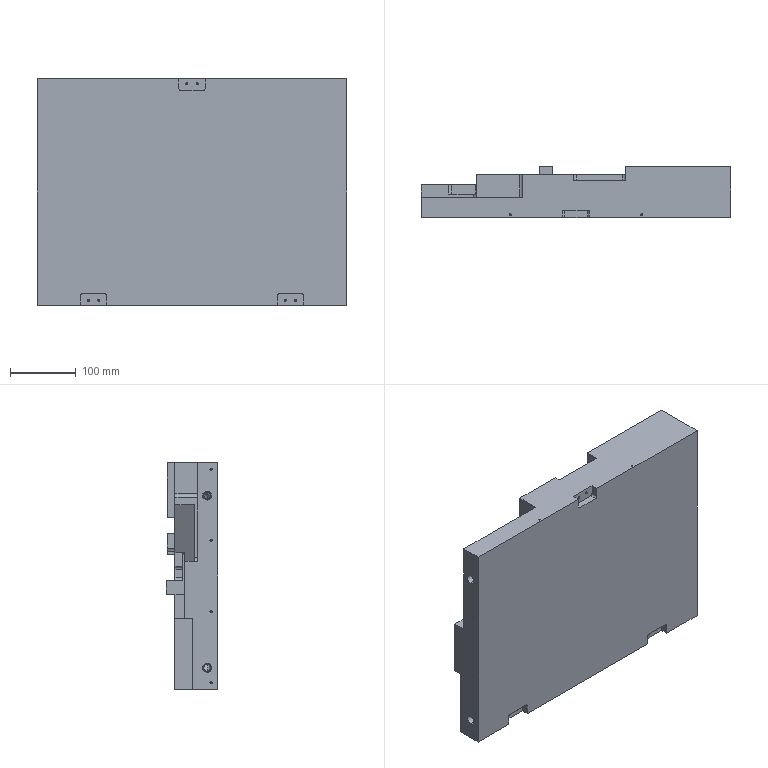Part | SolidWorks | features Cut 44, HoleWzd 43, MoveFace 39, ICE 30, DelFace 19, Fillet 18, MirrorPattern 5, SweepCut 2, Extrusion 1 | 1 solid | 679 faces | box 472 x 78 x 345 mm | volume 7845697 mm3 | cylinder 337 | cone 220 | plane 118 | torus 4 | commonest cylinder face diameters 2.5 x112 3.3 x76 2 x72 10 x27 1.6 x24 4 x12